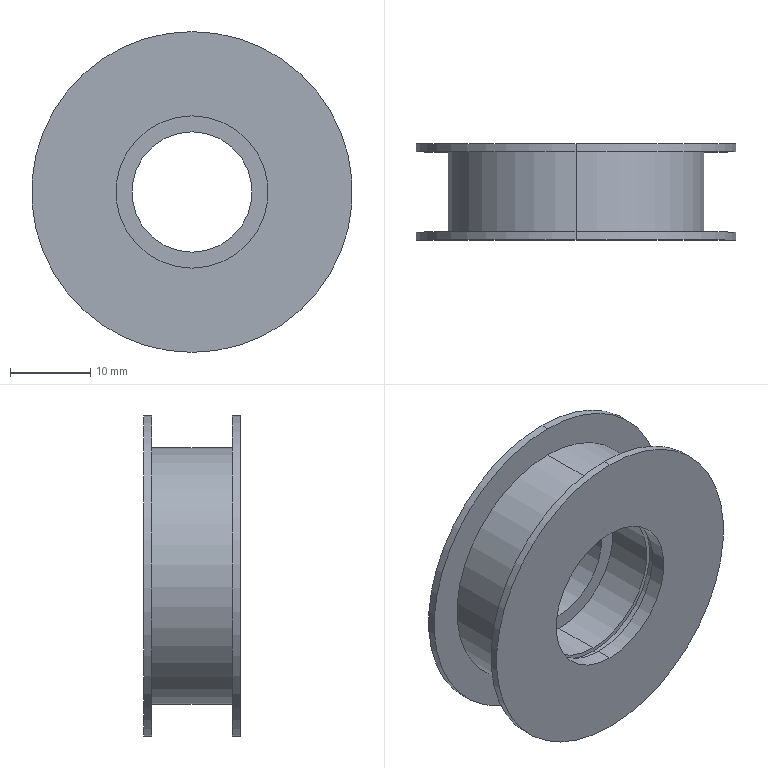Part | SolidWorks | features Revolution 1 | 1 solid | 21 faces | box 40 x 12 x 40 mm | volume 7443 mm3 | cylinder 14 | plane 7 | commonest cylinder face diameters 19 x4 40 x4 15 x2 20 x2 32 x2
STEP:
#1=CARTESIAN_POINT('',(0.,-9.,20.));
#2=VERTEX_POINT('',#1);
#3=CARTESIAN_POINT('',(0.,-9.,-20.));
#4=VERTEX_POINT('',#3);
#5=CARTESIAN_POINT('',(0.,-9.,0.));
#6=DIRECTION('',(0.,1.,0.));
#7=DIRECTION('',(0.,0.,1.));
#8=AXIS2_PLACEMENT_3D('',#5,#6,#7);
#9=CIRCLE('',#8,20.);
#10=EDGE_CURVE('',#2,#4,#9,.T.);
#11=ORIENTED_EDGE('',*,*,#10,.T.);
#12=CARTESIAN_POINT('',(0.,-8.,-20.));
#13=VERTEX_POINT('',#12);
#14=CARTESIAN_POINT('',(0.,22.495,-20.));
#15=DIRECTION('',(0.,1.,0.));
#16=VECTOR('',#15,1000.);
#17=LINE('',#14,#16);
#18=EDGE_CURVE('',#4,#13,#17,.T.);
#19=ORIENTED_EDGE('',*,*,#18,.T.);
#20=CARTESIAN_POINT('',(0.,-8.,20.));
#21=VERTEX_POINT('',#20);
#22=CARTESIAN_POINT('',(0.,-8.,0.));
#23=DIRECTION('',(0.,1.,0.));
#24=DIRECTION('',(0.,0.,1.));
#25=AXIS2_PLACEMENT_3D('',#22,#23,#24);
#26=CIRCLE('',#25,20.);
#27=EDGE_CURVE('',#21,#13,#26,.T.);
#28=ORIENTED_EDGE('',*,*,#27,.F.);
#29=CARTESIAN_POINT('',(0.,22.495,20.));
#30=DIRECTION('',(0.,1.,0.));
#31=VECTOR('',#30,1000.);
#32=LINE('',#29,#31);
#33=EDGE_CURVE('',#2,#21,#32,.T.);
#34=ORIENTED_EDGE('',*,*,#33,.F.);
#35=EDGE_LOOP('',(#11,#19,#28,#34));
#36=FACE_OUTER_BOUND('',#35,.T.);
#37=CARTESIAN_POINT('',(0.,22.495,0.));
#38=DIRECTION('',(0.,1.,0.));
#39=DIRECTION('',(0.,0.,1.));
#40=AXIS2_PLACEMENT_3D('',#37,#38,#39);
#41=CYLINDRICAL_SURFACE('',#40,20.);
#42=ADVANCED_FACE('',(#36),#41,.T.);
#43=CARTESIAN_POINT('',(0.,-9.,-9.5));
#44=VERTEX_POINT('',#43);
#45=CARTESIAN_POINT('',(0.,-9.,9.5));
#46=VERTEX_POINT('',#45);
#47=CARTESIAN_POINT('',(0.,-9.,0.));
#48=DIRECTION('',(0.,1.,0.));
#49=DIRECTION('',(0.,0.,1.));
#50=AXIS2_PLACEMENT_3D('',#47,#48,#49);
#51=CIRCLE('',#50,9.5);
#52=EDGE_CURVE('',#44,#46,#51,.T.);
#53=ORIENTED_EDGE('',*,*,#52,.F.);
#54=CARTESIAN_POINT('',(0.,-7.,-9.5));
#55=VERTEX_POINT('',#54);
#56=CARTESIAN_POINT('',(0.,22.495,-9.5));
#57=DIRECTION('',(0.,1.,0.));
#58=VECTOR('',#57,1000.);
#59=LINE('',#56,#58);
#60=EDGE_CURVE('',#44,#55,#59,.T.);
#61=ORIENTED_EDGE('',*,*,#60,.T.);
#62=CARTESIAN_POINT('',(0.,-7.,9.5));
#63=VERTEX_POINT('',#62);
#64=CARTESIAN_POINT('',(0.,-7.,0.));
#65=DIRECTION('',(0.,1.,0.));
#66=DIRECTION('',(0.,0.,1.));
#67=AXIS2_PLACEMENT_3D('',#64,#65,#66);
#68=CIRCLE('',#67,9.5);
#69=EDGE_CURVE('',#55,#63,#68,.T.);
#70=ORIENTED_EDGE('',*,*,#69,.T.);
#71=CARTESIAN_POINT('',(0.,22.495,9.5));
#72=DIRECTION('',(0.,1.,0.));
#73=VECTOR('',#72,1000.);
#74=LINE('',#71,#73);
#75=EDGE_CURVE('',#46,#63,#74,.T.);
#76=ORIENTED_EDGE('',*,*,#75,.F.);
#77=EDGE_LOOP('',(#53,#61,#70,#76));
#78=FACE_OUTER_BOUND('',#77,.T.);
#79=CARTESIAN_POINT('',(0.,22.495,0.));
#80=DIRECTION('',(0.,1.,0.));
#81=DIRECTION('',(0.,0.,1.));
#82=AXIS2_PLACEMENT_3D('',#79,#80,#81);
#83=CYLINDRICAL_SURFACE('',#82,9.5);
#84=ADVANCED_FACE('',(#78),#83,.F.);
#85=CARTESIAN_POINT('',(0.,-7.,-10.));
#86=VERTEX_POINT('',#85);
#87=CARTESIAN_POINT('',(0.,-7.,10.));
#88=VERTEX_POINT('',#87);
#89=CARTESIAN_POINT('',(0.,-7.,0.));
#90=DIRECTION('',(0.,1.,0.));
#91=DIRECTION('',(0.,0.,1.));
#92=AXIS2_PLACEMENT_3D('',#89,#90,#91);
#93=CIRCLE('',#92,10.);
#94=EDGE_CURVE('',#86,#88,#93,.T.);
#95=ORIENTED_EDGE('',*,*,#94,.F.);
#96=CARTESIAN_POINT('',(0.,-6.,-10.));
#97=VERTEX_POINT('',#96);
#98=CARTESIAN_POINT('',(0.,22.495,-10.));
#99=DIRECTION('',(0.,1.,0.));
#100=VECTOR('',#99,1000.);
#101=LINE('',#98,#100);
#102=EDGE_CURVE('',#86,#97,#101,.T.);
#103=ORIENTED_EDGE('',*,*,#102,.T.);
#104=CARTESIAN_POINT('',(0.,-6.,10.));
#105=VERTEX_POINT('',#104);
#106=CARTESIAN_POINT('',(0.,-6.,0.));
#107=DIRECTION('',(0.,1.,0.));
#108=DIRECTION('',(0.,0.,1.));
#109=AXIS2_PLACEMENT_3D('',#106,#107,#108);
#110=CIRCLE('',#109,10.);
#111=EDGE_CURVE('',#97,#105,#110,.T.);
#112=ORIENTED_EDGE('',*,*,#111,.T.);
#113=CARTESIAN_POINT('',(0.,22.495,10.));
#114=DIRECTION('',(0.,1.,0.));
#115=VECTOR('',#114,1000.);
#116=LINE('',#113,#115);
#117=EDGE_CURVE('',#88,#105,#116,.T.);
#118=ORIENTED_EDGE('',*,*,#117,.F.);
#119=EDGE_LOOP('',(#95,#103,#112,#118));
#120=FACE_OUTER_BOUND('',#119,.T.);
#121=CARTESIAN_POINT('',(0.,22.495,0.));
#122=DIRECTION('',(0.,1.,0.));
#123=DIRECTION('',(0.,0.,1.));
#124=AXIS2_PLACEMENT_3D('',#121,#122,#123);
#125=CYLINDRICAL_SURFACE('',#124,10.);
#126=ADVANCED_FACE('',(#120),#125,.F.);
#127=CARTESIAN_POINT('',(0.,-6.,-9.5));
#128=VERTEX_POINT('',#127);
#129=CARTESIAN_POINT('',(0.,-6.,9.5));
#130=VERTEX_POINT('',#129);
#131=CARTESIAN_POINT('',(0.,-6.,0.));
#132=DIRECTION('',(0.,1.,0.));
#133=DIRECTION('',(0.,0.,1.));
#134=AXIS2_PLACEMENT_3D('',#131,#132,#133);
#135=CIRCLE('',#134,9.5);
#136=EDGE_CURVE('',#128,#130,#135,.T.);
#137=ORIENTED_EDGE('',*,*,#136,.F.);
#138=CARTESIAN_POINT('',(0.,0.,-9.5));
#139=VERTEX_POINT('',#138);
#140=CARTESIAN_POINT('',(0.,22.495,-9.5));
#141=DIRECTION('',(0.,1.,0.));
#142=VECTOR('',#141,1000.);
#143=LINE('',#140,#142);
#144=EDGE_CURVE('',#128,#139,#143,.T.);
#145=ORIENTED_EDGE('',*,*,#144,.T.);
#146=CARTESIAN_POINT('',(0.,0.,9.5));
#147=VERTEX_POINT('',#146);
#148=CARTESIAN_POINT('',(0.,0.,0.));
#149=DIRECTION('',(0.,1.,0.));
#150=DIRECTION('',(0.,0.,1.));
#151=AXIS2_PLACEMENT_3D('',#148,#149,#150);
#152=CIRCLE('',#151,9.5);
#153=EDGE_CURVE('',#139,#147,#152,.T.);
#154=ORIENTED_EDGE('',*,*,#153,.T.);
#155=CARTESIAN_POINT('',(0.,22.495,9.5));
#156=DIRECTION('',(0.,1.,0.));
#157=VECTOR('',#156,1000.);
#158=LINE('',#155,#157);
#159=EDGE_CURVE('',#130,#147,#158,.T.);
#160=ORIENTED_EDGE('',*,*,#159,.F.);
#161=EDGE_LOOP('',(#137,#145,#154,#160));
#162=FACE_OUTER_BOUND('',#161,.T.);
#163=CARTESIAN_POINT('',(0.,22.495,0.));
#164=DIRECTION('',(0.,1.,0.));
#165=DIRECTION('',(0.,0.,1.));
#166=AXIS2_PLACEMENT_3D('',#163,#164,#165);
#167=CYLINDRICAL_SURFACE('',#166,9.5);
#168=ADVANCED_FACE('',(#162),#167,.F.);
#169=CARTESIAN_POINT('',(0.,0.,-7.5));
#170=VERTEX_POINT('',#169);
#171=CARTESIAN_POINT('',(0.,0.,7.5));
#172=VERTEX_POINT('',#171);
#173=CARTESIAN_POINT('',(0.,0.,0.));
#174=DIRECTION('',(0.,1.,0.));
#175=DIRECTION('',(0.,0.,1.));
#176=AXIS2_PLACEMENT_3D('',#173,#174,#175);
#177=CIRCLE('',#176,7.5);
#178=EDGE_CURVE('',#170,#172,#177,.T.);
#179=ORIENTED_EDGE('',*,*,#178,.F.);
#180=CARTESIAN_POINT('',(0.,3.,-7.5));
#181=VERTEX_POINT('',#180);
#182=CARTESIAN_POINT('',(0.,22.495,-7.5));
#183=DIRECTION('',(0.,1.,0.));
#184=VECTOR('',#183,1000.);
#185=LINE('',#182,#184);
#186=EDGE_CURVE('',#170,#181,#185,.T.);
#187=ORIENTED_EDGE('',*,*,#186,.T.);
#188=CARTESIAN_POINT('',(0.,3.,7.5));
#189=VERTEX_POINT('',#188);
#190=CARTESIAN_POINT('',(0.,3.,0.));
#191=DIRECTION('',(0.,1.,0.));
#192=DIRECTION('',(0.,0.,1.));
#193=AXIS2_PLACEMENT_3D('',#190,#191,#192);
#194=CIRCLE('',#193,7.5);
#195=EDGE_CURVE('',#181,#189,#194,.T.);
#196=ORIENTED_EDGE('',*,*,#195,.T.);
#197=CARTESIAN_POINT('',(0.,22.495,7.5));
#198=DIRECTION('',(0.,1.,0.));
#199=VECTOR('',#198,1000.);
#200=LINE('',#197,#199);
#201=EDGE_CURVE('',#172,#189,#200,.T.);
#202=ORIENTED_EDGE('',*,*,#201,.F.);
#203=EDGE_LOOP('',(#179,#187,#196,#202));
#204=FACE_OUTER_BOUND('',#203,.T.);
#205=CARTESIAN_POINT('',(0.,22.495,0.));
#206=DIRECTION('',(0.,1.,0.));
#207=DIRECTION('',(0.,0.,1.));
#208=AXIS2_PLACEMENT_3D('',#205,#206,#207);
#209=CYLINDRICAL_SURFACE('',#208,7.5);
#210=ADVANCED_FACE('',(#204),#209,.F.);
#211=CARTESIAN_POINT('',(0.,2.,20.));
#212=VERTEX_POINT('',#211);
#213=CARTESIAN_POINT('',(0.,2.,-20.));
#214=VERTEX_POINT('',#213);
#215=CARTESIAN_POINT('',(0.,2.,0.));
#216=DIRECTION('',(0.,1.,0.));
#217=DIRECTION('',(0.,0.,1.));
#218=AXIS2_PLACEMENT_3D('',#215,#216,#217);
#219=CIRCLE('',#218,20.);
#220=EDGE_CURVE('',#212,#214,#219,.T.);
#221=ORIENTED_EDGE('',*,*,#220,.T.);
#222=CARTESIAN_POINT('',(0.,3.,-20.));
#223=VERTEX_POINT('',#222);
#224=CARTESIAN_POINT('',(0.,22.495,-20.));
#225=DIRECTION('',(0.,1.,0.));
#226=VECTOR('',#225,1000.);
#227=LINE('',#224,#226);
#228=EDGE_CURVE('',#214,#223,#227,.T.);
#229=ORIENTED_EDGE('',*,*,#228,.T.);
#230=CARTESIAN_POINT('',(0.,3.,20.));
#231=VERTEX_POINT('',#230);
#232=CARTESIAN_POINT('',(0.,3.,0.));
#233=DIRECTION('',(0.,1.,0.));
#234=DIRECTION('',(0.,0.,1.));
#235=AXIS2_PLACEMENT_3D('',#232,#233,#234);
#236=CIRCLE('',#235,20.);
#237=EDGE_CURVE('',#231,#223,#236,.T.);
#238=ORIENTED_EDGE('',*,*,#237,.F.);
#239=CARTESIAN_POINT('',(0.,22.495,20.));
#240=DIRECTION('',(0.,1.,0.));
#241=VECTOR('',#240,1000.);
#242=LINE('',#239,#241);
#243=EDGE_CURVE('',#212,#231,#242,.T.);
#244=ORIENTED_EDGE('',*,*,#243,.F.);
#245=EDGE_LOOP('',(#221,#229,#238,#244));
#246=FACE_OUTER_BOUND('',#245,.T.);
#247=CARTESIAN_POINT('',(0.,22.495,0.));
#248=DIRECTION('',(0.,1.,0.));
#249=DIRECTION('',(0.,0.,1.));
#250=AXIS2_PLACEMENT_3D('',#247,#248,#249);
#251=CYLINDRICAL_SURFACE('',#250,20.);
#252=ADVANCED_FACE('',(#246),#251,.T.);
#253=CARTESIAN_POINT('',(0.,-8.,16.));
#254=VERTEX_POINT('',#253);
#255=CARTESIAN_POINT('',(0.,-8.,-16.));
#256=VERTEX_POINT('',#255);
#257=CARTESIAN_POINT('',(0.,-8.,0.));
#258=DIRECTION('',(0.,1.,0.));
#259=DIRECTION('',(0.,0.,1.));
#260=AXIS2_PLACEMENT_3D('',#257,#258,#259);
#261=CIRCLE('',#260,16.);
#262=EDGE_CURVE('',#254,#256,#261,.T.);
#263=ORIENTED_EDGE('',*,*,#262,.T.);
#264=CARTESIAN_POINT('',(0.,2.,-16.));
#265=VERTEX_POINT('',#264);
#266=CARTESIAN_POINT('',(0.,22.495,-16.));
#267=DIRECTION('',(0.,1.,0.));
#268=VECTOR('',#267,1000.);
#269=LINE('',#266,#268);
#270=EDGE_CURVE('',#256,#265,#269,.T.);
#271=ORIENTED_EDGE('',*,*,#270,.T.);
#272=CARTESIAN_POINT('',(0.,2.,16.));
#273=VERTEX_POINT('',#272);
#274=CARTESIAN_POINT('',(0.,2.,0.));
#275=DIRECTION('',(0.,1.,0.));
#276=DIRECTION('',(0.,0.,1.));
#277=AXIS2_PLACEMENT_3D('',#274,#275,#276);
#278=CIRCLE('',#277,16.);
#279=EDGE_CURVE('',#273,#265,#278,.T.);
#280=ORIENTED_EDGE('',*,*,#279,.F.);
#281=CARTESIAN_POINT('',(0.,22.495,16.));
#282=DIRECTION('',(0.,1.,0.));
#283=VECTOR('',#282,1000.);
#284=LINE('',#281,#283);
#285=EDGE_CURVE('',#254,#273,#284,.T.);
#286=ORIENTED_EDGE('',*,*,#285,.F.);
#287=EDGE_LOOP('',(#263,#271,#280,#286));
#288=FACE_OUTER_BOUND('',#287,.T.);
#289=CARTESIAN_POINT('',(0.,22.495,0.));
#290=DIRECTION('',(0.,1.,0.));
#291=DIRECTION('',(0.,0.,1.));
#292=AXIS2_PLACEMENT_3D('',#289,#290,#291);
#293=CYLINDRICAL_SURFACE('',#292,16.);
#294=ADVANCED_FACE('',(#288),#293,.T.);
#295=ORIENTED_EDGE('',*,*,#262,.F.);
#296=CARTESIAN_POINT('',(0.,-8.,0.));
#297=DIRECTION('',(0.,1.,0.));
#298=DIRECTION('',(0.,0.,1.));
#299=AXIS2_PLACEMENT_3D('',#296,#297,#298);
#300=CIRCLE('',#299,16.);
#301=EDGE_CURVE('',#256,#254,#300,.T.);
#302=ORIENTED_EDGE('',*,*,#301,.F.);
#303=EDGE_LOOP('',(#295,#302));
#304=FACE_BOUND('',#303,.T.);
#305=ORIENTED_EDGE('',*,*,#27,.T.);
#306=CARTESIAN_POINT('',(0.,-8.,0.));
#307=DIRECTION('',(0.,1.,0.));
#308=DIRECTION('',(0.,0.,1.));
#309=AXIS2_PLACEMENT_3D('',#306,#307,#308);
#310=CIRCLE('',#309,20.);
#311=EDGE_CURVE('',#13,#21,#310,.T.);
#312=ORIENTED_EDGE('',*,*,#311,.T.);
#313=EDGE_LOOP('',(#305,#312));
#314=FACE_OUTER_BOUND('',#313,.T.);
#315=CARTESIAN_POINT('',(16.,-8.,0.));
#316=DIRECTION('',(0.,-1.,0.));
#317=DIRECTION('',(0.,0.,-1.));
#318=AXIS2_PLACEMENT_3D('',#315,#316,#317);
#319=PLANE('',#318);
#320=ADVANCED_FACE('',(#304,#314),#319,.F.);
#321=ORIENTED_EDGE('',*,*,#270,.F.);
#322=ORIENTED_EDGE('',*,*,#301,.T.);
#323=ORIENTED_EDGE('',*,*,#285,.T.);
#324=CARTESIAN_POINT('',(0.,2.,0.));
#325=DIRECTION('',(0.,1.,0.));
#326=DIRECTION('',(0.,0.,1.));
#327=AXIS2_PLACEMENT_3D('',#324,#325,#326);
#328=CIRCLE('',#327,16.);
#329=EDGE_CURVE('',#265,#273,#328,.T.);
#330=ORIENTED_EDGE('',*,*,#329,.F.);
#331=EDGE_LOOP('',(#321,#322,#323,#330));
#332=FACE_OUTER_BOUND('',#331,.T.);
#333=CARTESIAN_POINT('',(0.,22.495,0.));
#334=DIRECTION('',(0.,1.,0.));
#335=DIRECTION('',(0.,0.,1.));
#336=AXIS2_PLACEMENT_3D('',#333,#334,#335);
#337=CYLINDRICAL_SURFACE('',#336,16.);
#338=ADVANCED_FACE('',(#332),#337,.T.);
#339=ORIENTED_EDGE('',*,*,#220,.F.);
#340=CARTESIAN_POINT('',(0.,2.,0.));
#341=DIRECTION('',(0.,1.,0.));
#342=DIRECTION('',(0.,0.,1.));
#343=AXIS2_PLACEMENT_3D('',#340,#341,#342);
#344=CIRCLE('',#343,20.);
#345=EDGE_CURVE('',#214,#212,#344,.T.);
#346=ORIENTED_EDGE('',*,*,#345,.F.);
#347=EDGE_LOOP('',(#339,#346));
#348=FACE_OUTER_BOUND('',#347,.T.);
#349=ORIENTED_EDGE('',*,*,#279,.T.);
#350=ORIENTED_EDGE('',*,*,#329,.T.);
#351=EDGE_LOOP('',(#349,#350));
#352=FACE_BOUND('',#351,.T.);
#353=CARTESIAN_POINT('',(20.,2.,0.));
#354=DIRECTION('',(0.,1.,0.));
#355=DIRECTION('',(0.,0.,1.));
#356=AXIS2_PLACEMENT_3D('',#353,#354,#355);
#357=PLANE('',#356);
#358=ADVANCED_FACE('',(#348,#352),#357,.F.);
#359=ORIENTED_EDGE('',*,*,#228,.F.);
#360=ORIENTED_EDGE('',*,*,#345,.T.);
#361=ORIENTED_EDGE('',*,*,#243,.T.);
#362=CARTESIAN_POINT('',(0.,3.,0.));
#363=DIRECTION('',(0.,1.,0.));
#364=DIRECTION('',(0.,0.,1.));
#365=AXIS2_PLACEMENT_3D('',#362,#363,#364);
#366=CIRCLE('',#365,20.);
#367=EDGE_CURVE('',#223,#231,#366,.T.);
#368=ORIENTED_EDGE('',*,*,#367,.F.);
#369=EDGE_LOOP('',(#359,#360,#361,#368));
#370=FACE_OUTER_BOUND('',#369,.T.);
#371=CARTESIAN_POINT('',(0.,22.495,0.));
#372=DIRECTION('',(0.,1.,0.));
#373=DIRECTION('',(0.,0.,1.));
#374=AXIS2_PLACEMENT_3D('',#371,#372,#373);
#375=CYLINDRICAL_SURFACE('',#374,20.);
#376=ADVANCED_FACE('',(#370),#375,.T.);
#377=CARTESIAN_POINT('',(0.,3.,0.));
#378=DIRECTION('',(0.,1.,0.));
#379=DIRECTION('',(0.,0.,1.));
#380=AXIS2_PLACEMENT_3D('',#377,#378,#379);
#381=CIRCLE('',#380,7.5);
#382=EDGE_CURVE('',#189,#181,#381,.T.);
#383=ORIENTED_EDGE('',*,*,#382,.F.);
#384=ORIENTED_EDGE('',*,*,#195,.F.);
#385=EDGE_LOOP('',(#383,#384));
#386=FACE_BOUND('',#385,.T.);
#387=ORIENTED_EDGE('',*,*,#237,.T.);
#388=ORIENTED_EDGE('',*,*,#367,.T.);
#389=EDGE_LOOP('',(#387,#388));
#390=FACE_OUTER_BOUND('',#389,.T.);
#391=CARTESIAN_POINT('',(20.,3.,0.));
#392=DIRECTION('',(0.,-1.,0.));
#393=DIRECTION('',(0.,0.,-1.));
#394=AXIS2_PLACEMENT_3D('',#391,#392,#393);
#395=PLANE('',#394);
#396=ADVANCED_FACE('',(#386,#390),#395,.F.);
#397=ORIENTED_EDGE('',*,*,#186,.F.);
#398=CARTESIAN_POINT('',(0.,0.,0.));
#399=DIRECTION('',(0.,1.,0.));
#400=DIRECTION('',(0.,0.,1.));
#401=AXIS2_PLACEMENT_3D('',#398,#399,#400);
#402=CIRCLE('',#401,7.5);
#403=EDGE_CURVE('',#172,#170,#402,.T.);
#404=ORIENTED_EDGE('',*,*,#403,.F.);
#405=ORIENTED_EDGE('',*,*,#201,.T.);
#406=ORIENTED_EDGE('',*,*,#382,.T.);
#407=EDGE_LOOP('',(#397,#404,#405,#406));
#408=FACE_OUTER_BOUND('',#407,.T.);
#409=CARTESIAN_POINT('',(0.,22.495,0.));
#410=DIRECTION('',(0.,1.,0.));
#411=DIRECTION('',(0.,0.,1.));
#412=AXIS2_PLACEMENT_3D('',#409,#410,#411);
#413=CYLINDRICAL_SURFACE('',#412,7.5);
#414=ADVANCED_FACE('',(#408),#413,.F.);
#415=CARTESIAN_POINT('',(0.,0.,0.));
#416=DIRECTION('',(0.,1.,0.));
#417=DIRECTION('',(0.,0.,1.));
#418=AXIS2_PLACEMENT_3D('',#415,#416,#417);
#419=CIRCLE('',#418,9.5);
#420=EDGE_CURVE('',#147,#139,#419,.T.);
#421=ORIENTED_EDGE('',*,*,#420,.F.);
#422=ORIENTED_EDGE('',*,*,#153,.F.);
#423=EDGE_LOOP('',(#421,#422));
#424=FACE_OUTER_BOUND('',#423,.T.);
#425=ORIENTED_EDGE('',*,*,#403,.T.);
#426=ORIENTED_EDGE('',*,*,#178,.T.);
#427=EDGE_LOOP('',(#425,#426));
#428=FACE_BOUND('',#427,.T.);
#429=CARTESIAN_POINT('',(7.5,0.,0.));
#430=DIRECTION('',(0.,1.,0.));
#431=DIRECTION('',(0.,0.,1.));
#432=AXIS2_PLACEMENT_3D('',#429,#430,#431);
#433=PLANE('',#432);
#434=ADVANCED_FACE('',(#424,#428),#433,.F.);
#435=ORIENTED_EDGE('',*,*,#144,.F.);
#436=CARTESIAN_POINT('',(0.,-6.,0.));
#437=DIRECTION('',(0.,1.,0.));
#438=DIRECTION('',(0.,0.,1.));
#439=AXIS2_PLACEMENT_3D('',#436,#437,#438);
#440=CIRCLE('',#439,9.5);
#441=EDGE_CURVE('',#130,#128,#440,.T.);
#442=ORIENTED_EDGE('',*,*,#441,.F.);
#443=ORIENTED_EDGE('',*,*,#159,.T.);
#444=ORIENTED_EDGE('',*,*,#420,.T.);
#445=EDGE_LOOP('',(#435,#442,#443,#444));
#446=FACE_OUTER_BOUND('',#445,.T.);
#447=CARTESIAN_POINT('',(0.,22.495,0.));
#448=DIRECTION('',(0.,1.,0.));
#449=DIRECTION('',(0.,0.,1.));
#450=AXIS2_PLACEMENT_3D('',#447,#448,#449);
#451=CYLINDRICAL_SURFACE('',#450,9.5);
#452=ADVANCED_FACE('',(#446),#451,.F.);
#453=CARTESIAN_POINT('',(0.,-6.,0.));
#454=DIRECTION('',(0.,1.,0.));
#455=DIRECTION('',(0.,0.,1.));
#456=AXIS2_PLACEMENT_3D('',#453,#454,#455);
#457=CIRCLE('',#456,10.);
#458=EDGE_CURVE('',#105,#97,#457,.T.);
#459=ORIENTED_EDGE('',*,*,#458,.F.);
#460=ORIENTED_EDGE('',*,*,#111,.F.);
#461=EDGE_LOOP('',(#459,#460));
#462=FACE_OUTER_BOUND('',#461,.T.);
#463=ORIENTED_EDGE('',*,*,#441,.T.);
#464=ORIENTED_EDGE('',*,*,#136,.T.);
#465=EDGE_LOOP('',(#463,#464));
#466=FACE_BOUND('',#465,.T.);
#467=CARTESIAN_POINT('',(10.,-6.,0.));
#468=DIRECTION('',(0.,1.,0.));
#469=DIRECTION('',(0.,0.,1.));
#470=AXIS2_PLACEMENT_3D('',#467,#468,#469);
#471=PLANE('',#470);
#472=ADVANCED_FACE('',(#462,#466),#471,.F.);
#473=ORIENTED_EDGE('',*,*,#102,.F.);
#474=CARTESIAN_POINT('',(0.,-7.,0.));
#475=DIRECTION('',(0.,1.,0.));
#476=DIRECTION('',(0.,0.,1.));
#477=AXIS2_PLACEMENT_3D('',#474,#475,#476);
#478=CIRCLE('',#477,10.);
#479=EDGE_CURVE('',#88,#86,#478,.T.);
#480=ORIENTED_EDGE('',*,*,#479,.F.);
#481=ORIENTED_EDGE('',*,*,#117,.T.);
#482=ORIENTED_EDGE('',*,*,#458,.T.);
#483=EDGE_LOOP('',(#473,#480,#481,#482));
#484=FACE_OUTER_BOUND('',#483,.T.);
#485=CARTESIAN_POINT('',(0.,22.495,0.));
#486=DIRECTION('',(0.,1.,0.));
#487=DIRECTION('',(0.,0.,1.));
#488=AXIS2_PLACEMENT_3D('',#485,#486,#487);
#489=CYLINDRICAL_SURFACE('',#488,10.);
#490=ADVANCED_FACE('',(#484),#489,.F.);
#491=CARTESIAN_POINT('',(0.,-7.,0.));
#492=DIRECTION('',(0.,1.,0.));
#493=DIRECTION('',(0.,0.,1.));
#494=AXIS2_PLACEMENT_3D('',#491,#492,#493);
#495=CIRCLE('',#494,9.5);
#496=EDGE_CURVE('',#63,#55,#495,.T.);
#497=ORIENTED_EDGE('',*,*,#496,.F.);
#498=ORIENTED_EDGE('',*,*,#69,.F.);
#499=EDGE_LOOP('',(#497,#498));
#500=FACE_BOUND('',#499,.T.);
#501=ORIENTED_EDGE('',*,*,#479,.T.);
#502=ORIENTED_EDGE('',*,*,#94,.T.);
#503=EDGE_LOOP('',(#501,#502));
#504=FACE_OUTER_BOUND('',#503,.T.);
#505=CARTESIAN_POINT('',(9.5,-7.,0.));
#506=DIRECTION('',(0.,-1.,0.));
#507=DIRECTION('',(0.,0.,-1.));
#508=AXIS2_PLACEMENT_3D('',#505,#506,#507);
#509=PLANE('',#508);
#510=ADVANCED_FACE('',(#500,#504),#509,.F.);
#511=ORIENTED_EDGE('',*,*,#60,.F.);
#512=CARTESIAN_POINT('',(0.,-9.,0.));
#513=DIRECTION('',(0.,1.,0.));
#514=DIRECTION('',(0.,0.,1.));
#515=AXIS2_PLACEMENT_3D('',#512,#513,#514);
#516=CIRCLE('',#515,9.5);
#517=EDGE_CURVE('',#46,#44,#516,.T.);
#518=ORIENTED_EDGE('',*,*,#517,.F.);
#519=ORIENTED_EDGE('',*,*,#75,.T.);
#520=ORIENTED_EDGE('',*,*,#496,.T.);
#521=EDGE_LOOP('',(#511,#518,#519,#520));
#522=FACE_OUTER_BOUND('',#521,.T.);
#523=CARTESIAN_POINT('',(0.,22.495,0.));
#524=DIRECTION('',(0.,1.,0.));
#525=DIRECTION('',(0.,0.,1.));
#526=AXIS2_PLACEMENT_3D('',#523,#524,#525);
#527=CYLINDRICAL_SURFACE('',#526,9.5);
#528=ADVANCED_FACE('',(#522),#527,.F.);
#529=ORIENTED_EDGE('',*,*,#10,.F.);
#530=CARTESIAN_POINT('',(0.,-9.,0.));
#531=DIRECTION('',(0.,1.,0.));
#532=DIRECTION('',(0.,0.,1.));
#533=AXIS2_PLACEMENT_3D('',#530,#531,#532);
#534=CIRCLE('',#533,20.);
#535=EDGE_CURVE('',#4,#2,#534,.T.);
#536=ORIENTED_EDGE('',*,*,#535,.F.);
#537=EDGE_LOOP('',(#529,#536));
#538=FACE_OUTER_BOUND('',#537,.T.);
#539=ORIENTED_EDGE('',*,*,#517,.T.);
#540=ORIENTED_EDGE('',*,*,#52,.T.);
#541=EDGE_LOOP('',(#539,#540));
#542=FACE_BOUND('',#541,.T.);
#543=CARTESIAN_POINT('',(9.5,-9.,0.));
#544=DIRECTION('',(0.,1.,0.));
#545=DIRECTION('',(0.,0.,1.));
#546=AXIS2_PLACEMENT_3D('',#543,#544,#545);
#547=PLANE('',#546);
#548=ADVANCED_FACE('',(#538,#542),#547,.F.);
#549=ORIENTED_EDGE('',*,*,#18,.F.);
#550=ORIENTED_EDGE('',*,*,#535,.T.);
#551=ORIENTED_EDGE('',*,*,#33,.T.);
#552=ORIENTED_EDGE('',*,*,#311,.F.);
#553=EDGE_LOOP('',(#549,#550,#551,#552));
#554=FACE_OUTER_BOUND('',#553,.T.);
#555=CARTESIAN_POINT('',(0.,22.495,0.));
#556=DIRECTION('',(0.,1.,0.));
#557=DIRECTION('',(0.,0.,1.));
#558=AXIS2_PLACEMENT_3D('',#555,#556,#557);
#559=CYLINDRICAL_SURFACE('',#558,20.);
#560=ADVANCED_FACE('',(#554),#559,.T.);
#561=CLOSED_SHELL('',(#42,#84,#126,#168,#210,#252,#294,#320,#338,#358,#376,#396,#414,#434,#452,#472,#490,#510,#528,#548,#560));
#562=MANIFOLD_SOLID_BREP('',#561);
#563=CARTESIAN_POINT('',(0.,0.,0.));
#564=DIRECTION('',(0.,0.,1.));
#565=DIRECTION('',(1.,0.,0.));
#566=AXIS2_PLACEMENT_3D('',#563,#564,#565);
#567=(LENGTH_UNIT()NAMED_UNIT(*)SI_UNIT(.MILLI.,.METRE.));
#568=UNCERTAINTY_MEASURE_WITH_UNIT(LENGTH_MEASURE(0.00001),#567,'','');
#569=(NAMED_UNIT(*)PLANE_ANGLE_UNIT()SI_UNIT($,.RADIAN.));
#570=(NAMED_UNIT(*)SI_UNIT($,.STERADIAN.)SOLID_ANGLE_UNIT());
#571=(GEOMETRIC_REPRESENTATION_CONTEXT(3)GLOBAL_UNCERTAINTY_ASSIGNED_CONTEXT((#568))GLOBAL_UNIT_ASSIGNED_CONTEXT((#567,#569,#570))REPRESENTATION_CONTEXT('',''));
#572=ADVANCED_BREP_SHAPE_REPRESENTATION('',(#562,#566),#571);